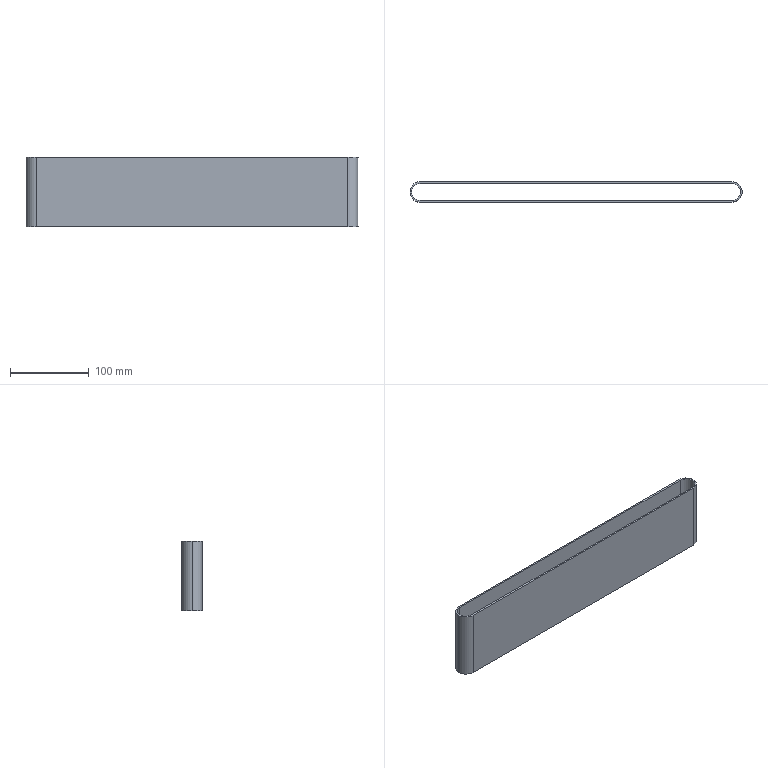Part | STEP file | Red flat belt 816 | 1 solid | 12 faces | box 423 x 26 x 89 mm | volume 154753 mm3 | cylinder 6 | plane 6 | commonest cylinder face diameters 22 x3 26 x3
STEP:
#1=CARTESIAN_POINT('',(-198.5,11.,89.));
#2=VERTEX_POINT('',#1);
#3=CARTESIAN_POINT('',(-209.5,0.,89.));
#4=VERTEX_POINT('',#3);
#5=CARTESIAN_POINT('',(-198.5,0.,89.));
#6=DIRECTION('',(0.,0.,1.));
#7=DIRECTION('',(1.,0.,0.));
#8=AXIS2_PLACEMENT_3D('',#5,#6,#7);
#9=CIRCLE('',#8,11.);
#10=EDGE_CURVE('',#2,#4,#9,.T.);
#11=ORIENTED_EDGE('',*,*,#10,.T.);
#12=CARTESIAN_POINT('',(-209.5,0.,0.));
#13=VERTEX_POINT('',#12);
#14=CARTESIAN_POINT('',(-209.5,0.,89.));
#15=DIRECTION('',(0.,0.,-1.));
#16=VECTOR('',#15,1000.);
#17=LINE('',#14,#16);
#18=EDGE_CURVE('',#4,#13,#17,.T.);
#19=ORIENTED_EDGE('',*,*,#18,.T.);
#20=CARTESIAN_POINT('',(-198.5,11.,0.));
#21=VERTEX_POINT('',#20);
#22=CARTESIAN_POINT('',(-198.5,0.,0.));
#23=DIRECTION('',(0.,0.,1.));
#24=DIRECTION('',(1.,0.,0.));
#25=AXIS2_PLACEMENT_3D('',#22,#23,#24);
#26=CIRCLE('',#25,11.);
#27=EDGE_CURVE('',#21,#13,#26,.T.);
#28=ORIENTED_EDGE('',*,*,#27,.F.);
#29=CARTESIAN_POINT('',(-198.5,11.,89.));
#30=DIRECTION('',(0.,0.,-1.));
#31=VECTOR('',#30,1000.);
#32=LINE('',#29,#31);
#33=EDGE_CURVE('',#2,#21,#32,.T.);
#34=ORIENTED_EDGE('',*,*,#33,.F.);
#35=EDGE_LOOP('',(#11,#19,#28,#34));
#36=FACE_OUTER_BOUND('',#35,.T.);
#37=CARTESIAN_POINT('',(-198.5,0.,89.));
#38=DIRECTION('',(0.,0.,-1.));
#39=DIRECTION('',(-1.,0.,0.));
#40=AXIS2_PLACEMENT_3D('',#37,#38,#39);
#41=CYLINDRICAL_SURFACE('',#40,11.);
#42=ADVANCED_FACE('',(#36),#41,.F.);
#43=CARTESIAN_POINT('',(-211.5,0.,89.));
#44=VERTEX_POINT('',#43);
#45=CARTESIAN_POINT('',(-198.5,-13.,89.));
#46=VERTEX_POINT('',#45);
#47=CARTESIAN_POINT('',(-198.5,0.,89.));
#48=DIRECTION('',(0.,0.,1.));
#49=DIRECTION('',(1.,0.,0.));
#50=AXIS2_PLACEMENT_3D('',#47,#48,#49);
#51=CIRCLE('',#50,13.);
#52=EDGE_CURVE('',#44,#46,#51,.T.);
#53=ORIENTED_EDGE('',*,*,#52,.F.);
#54=CARTESIAN_POINT('',(-211.5,0.,0.));
#55=VERTEX_POINT('',#54);
#56=CARTESIAN_POINT('',(-211.5,0.,89.));
#57=DIRECTION('',(0.,0.,-1.));
#58=VECTOR('',#57,1000.);
#59=LINE('',#56,#58);
#60=EDGE_CURVE('',#44,#55,#59,.T.);
#61=ORIENTED_EDGE('',*,*,#60,.T.);
#62=CARTESIAN_POINT('',(-198.5,-13.,0.));
#63=VERTEX_POINT('',#62);
#64=CARTESIAN_POINT('',(-198.5,0.,0.));
#65=DIRECTION('',(0.,0.,1.));
#66=DIRECTION('',(1.,0.,0.));
#67=AXIS2_PLACEMENT_3D('',#64,#65,#66);
#68=CIRCLE('',#67,13.);
#69=EDGE_CURVE('',#55,#63,#68,.T.);
#70=ORIENTED_EDGE('',*,*,#69,.T.);
#71=CARTESIAN_POINT('',(-198.5,-13.,89.));
#72=DIRECTION('',(0.,0.,-1.));
#73=VECTOR('',#72,1000.);
#74=LINE('',#71,#73);
#75=EDGE_CURVE('',#46,#63,#74,.T.);
#76=ORIENTED_EDGE('',*,*,#75,.F.);
#77=EDGE_LOOP('',(#53,#61,#70,#76));
#78=FACE_OUTER_BOUND('',#77,.T.);
#79=CARTESIAN_POINT('',(-198.5,0.,89.));
#80=DIRECTION('',(0.,0.,-1.));
#81=DIRECTION('',(-1.,0.,0.));
#82=AXIS2_PLACEMENT_3D('',#79,#80,#81);
#83=CYLINDRICAL_SURFACE('',#82,13.);
#84=ADVANCED_FACE('',(#78),#83,.T.);
#85=CARTESIAN_POINT('',(-198.5,13.,89.));
#86=VERTEX_POINT('',#85);
#87=CARTESIAN_POINT('',(-198.5,0.,89.));
#88=DIRECTION('',(0.,0.,1.));
#89=DIRECTION('',(1.,0.,0.));
#90=AXIS2_PLACEMENT_3D('',#87,#88,#89);
#91=CIRCLE('',#90,13.);
#92=EDGE_CURVE('',#86,#44,#91,.T.);
#93=ORIENTED_EDGE('',*,*,#92,.T.);
#94=ORIENTED_EDGE('',*,*,#52,.T.);
#95=CARTESIAN_POINT('',(198.5,-13.,89.));
#96=VERTEX_POINT('',#95);
#97=CARTESIAN_POINT('',(-198.5,-13.,89.));
#98=DIRECTION('',(1.,0.,0.));
#99=VECTOR('',#98,1000.);
#100=LINE('',#97,#99);
#101=EDGE_CURVE('',#46,#96,#100,.T.);
#102=ORIENTED_EDGE('',*,*,#101,.T.);
#103=CARTESIAN_POINT('',(198.5,13.,89.));
#104=VERTEX_POINT('',#103);
#105=CARTESIAN_POINT('',(198.5,0.,89.));
#106=DIRECTION('',(0.,0.,1.));
#107=DIRECTION('',(1.,0.,0.));
#108=AXIS2_PLACEMENT_3D('',#105,#106,#107);
#109=CIRCLE('',#108,13.);
#110=EDGE_CURVE('',#96,#104,#109,.T.);
#111=ORIENTED_EDGE('',*,*,#110,.T.);
#112=CARTESIAN_POINT('',(-198.5,13.,89.));
#113=DIRECTION('',(-1.,0.,0.));
#114=VECTOR('',#113,1000.);
#115=LINE('',#112,#114);
#116=EDGE_CURVE('',#104,#86,#115,.T.);
#117=ORIENTED_EDGE('',*,*,#116,.T.);
#118=EDGE_LOOP('',(#93,#94,#102,#111,#117));
#119=FACE_OUTER_BOUND('',#118,.T.);
#120=CARTESIAN_POINT('',(-198.5,-11.,89.));
#121=VERTEX_POINT('',#120);
#122=CARTESIAN_POINT('',(198.5,-11.,89.));
#123=VERTEX_POINT('',#122);
#124=CARTESIAN_POINT('',(-198.5,-11.,89.));
#125=DIRECTION('',(1.,0.,0.));
#126=VECTOR('',#125,1000.);
#127=LINE('',#124,#126);
#128=EDGE_CURVE('',#121,#123,#127,.T.);
#129=ORIENTED_EDGE('',*,*,#128,.F.);
#130=CARTESIAN_POINT('',(-198.5,0.,89.));
#131=DIRECTION('',(0.,0.,1.));
#132=DIRECTION('',(1.,0.,0.));
#133=AXIS2_PLACEMENT_3D('',#130,#131,#132);
#134=CIRCLE('',#133,11.);
#135=EDGE_CURVE('',#4,#121,#134,.T.);
#136=ORIENTED_EDGE('',*,*,#135,.F.);
#137=ORIENTED_EDGE('',*,*,#10,.F.);
#138=CARTESIAN_POINT('',(198.5,11.,89.));
#139=VERTEX_POINT('',#138);
#140=CARTESIAN_POINT('',(-198.5,11.,89.));
#141=DIRECTION('',(-1.,0.,0.));
#142=VECTOR('',#141,1000.);
#143=LINE('',#140,#142);
#144=EDGE_CURVE('',#139,#2,#143,.T.);
#145=ORIENTED_EDGE('',*,*,#144,.F.);
#146=CARTESIAN_POINT('',(198.5,0.,89.));
#147=DIRECTION('',(0.,0.,1.));
#148=DIRECTION('',(1.,0.,0.));
#149=AXIS2_PLACEMENT_3D('',#146,#147,#148);
#150=CIRCLE('',#149,11.);
#151=EDGE_CURVE('',#123,#139,#150,.T.);
#152=ORIENTED_EDGE('',*,*,#151,.F.);
#153=EDGE_LOOP('',(#129,#136,#137,#145,#152));
#154=FACE_BOUND('',#153,.T.);
#155=CARTESIAN_POINT('',(-198.5,0.,89.));
#156=DIRECTION('',(0.,0.,1.));
#157=DIRECTION('',(1.,0.,0.));
#158=AXIS2_PLACEMENT_3D('',#155,#156,#157);
#159=PLANE('',#158);
#160=ADVANCED_FACE('',(#119,#154),#159,.T.);
#161=CARTESIAN_POINT('',(-198.5,13.,0.));
#162=VERTEX_POINT('',#161);
#163=CARTESIAN_POINT('',(-198.5,0.,0.));
#164=DIRECTION('',(0.,0.,1.));
#165=DIRECTION('',(1.,0.,0.));
#166=AXIS2_PLACEMENT_3D('',#163,#164,#165);
#167=CIRCLE('',#166,13.);
#168=EDGE_CURVE('',#162,#55,#167,.T.);
#169=ORIENTED_EDGE('',*,*,#168,.F.);
#170=CARTESIAN_POINT('',(198.5,13.,0.));
#171=VERTEX_POINT('',#170);
#172=CARTESIAN_POINT('',(-198.5,13.,0.));
#173=DIRECTION('',(-1.,0.,0.));
#174=VECTOR('',#173,1000.);
#175=LINE('',#172,#174);
#176=EDGE_CURVE('',#171,#162,#175,.T.);
#177=ORIENTED_EDGE('',*,*,#176,.F.);
#178=CARTESIAN_POINT('',(198.5,-13.,0.));
#179=VERTEX_POINT('',#178);
#180=CARTESIAN_POINT('',(198.5,0.,0.));
#181=DIRECTION('',(0.,0.,1.));
#182=DIRECTION('',(1.,0.,0.));
#183=AXIS2_PLACEMENT_3D('',#180,#181,#182);
#184=CIRCLE('',#183,13.);
#185=EDGE_CURVE('',#179,#171,#184,.T.);
#186=ORIENTED_EDGE('',*,*,#185,.F.);
#187=CARTESIAN_POINT('',(-198.5,-13.,0.));
#188=DIRECTION('',(1.,0.,0.));
#189=VECTOR('',#188,1000.);
#190=LINE('',#187,#189);
#191=EDGE_CURVE('',#63,#179,#190,.T.);
#192=ORIENTED_EDGE('',*,*,#191,.F.);
#193=ORIENTED_EDGE('',*,*,#69,.F.);
#194=EDGE_LOOP('',(#169,#177,#186,#192,#193));
#195=FACE_OUTER_BOUND('',#194,.T.);
#196=ORIENTED_EDGE('',*,*,#27,.T.);
#197=CARTESIAN_POINT('',(-198.5,-11.,0.));
#198=VERTEX_POINT('',#197);
#199=CARTESIAN_POINT('',(-198.5,0.,0.));
#200=DIRECTION('',(0.,0.,1.));
#201=DIRECTION('',(1.,0.,0.));
#202=AXIS2_PLACEMENT_3D('',#199,#200,#201);
#203=CIRCLE('',#202,11.);
#204=EDGE_CURVE('',#13,#198,#203,.T.);
#205=ORIENTED_EDGE('',*,*,#204,.T.);
#206=CARTESIAN_POINT('',(198.5,-11.,0.));
#207=VERTEX_POINT('',#206);
#208=CARTESIAN_POINT('',(-198.5,-11.,0.));
#209=DIRECTION('',(1.,0.,0.));
#210=VECTOR('',#209,1000.);
#211=LINE('',#208,#210);
#212=EDGE_CURVE('',#198,#207,#211,.T.);
#213=ORIENTED_EDGE('',*,*,#212,.T.);
#214=CARTESIAN_POINT('',(198.5,11.,0.));
#215=VERTEX_POINT('',#214);
#216=CARTESIAN_POINT('',(198.5,0.,0.));
#217=DIRECTION('',(0.,0.,1.));
#218=DIRECTION('',(1.,0.,0.));
#219=AXIS2_PLACEMENT_3D('',#216,#217,#218);
#220=CIRCLE('',#219,11.);
#221=EDGE_CURVE('',#207,#215,#220,.T.);
#222=ORIENTED_EDGE('',*,*,#221,.T.);
#223=CARTESIAN_POINT('',(-198.5,11.,0.));
#224=DIRECTION('',(-1.,0.,0.));
#225=VECTOR('',#224,1000.);
#226=LINE('',#223,#225);
#227=EDGE_CURVE('',#215,#21,#226,.T.);
#228=ORIENTED_EDGE('',*,*,#227,.T.);
#229=EDGE_LOOP('',(#196,#205,#213,#222,#228));
#230=FACE_BOUND('',#229,.T.);
#231=CARTESIAN_POINT('',(-198.5,0.,0.));
#232=DIRECTION('',(0.,0.,1.));
#233=DIRECTION('',(1.,0.,0.));
#234=AXIS2_PLACEMENT_3D('',#231,#232,#233);
#235=PLANE('',#234);
#236=ADVANCED_FACE('',(#195,#230),#235,.F.);
#237=ORIENTED_EDGE('',*,*,#60,.F.);
#238=ORIENTED_EDGE('',*,*,#92,.F.);
#239=CARTESIAN_POINT('',(-198.5,13.,89.));
#240=DIRECTION('',(0.,0.,-1.));
#241=VECTOR('',#240,1000.);
#242=LINE('',#239,#241);
#243=EDGE_CURVE('',#86,#162,#242,.T.);
#244=ORIENTED_EDGE('',*,*,#243,.T.);
#245=ORIENTED_EDGE('',*,*,#168,.T.);
#246=EDGE_LOOP('',(#237,#238,#244,#245));
#247=FACE_OUTER_BOUND('',#246,.T.);
#248=CARTESIAN_POINT('',(-198.5,0.,89.));
#249=DIRECTION('',(0.,0.,-1.));
#250=DIRECTION('',(-1.,0.,0.));
#251=AXIS2_PLACEMENT_3D('',#248,#249,#250);
#252=CYLINDRICAL_SURFACE('',#251,13.);
#253=ADVANCED_FACE('',(#247),#252,.T.);
#254=ORIENTED_EDGE('',*,*,#191,.T.);
#255=CARTESIAN_POINT('',(198.5,-13.,89.));
#256=DIRECTION('',(0.,0.,-1.));
#257=VECTOR('',#256,1000.);
#258=LINE('',#255,#257);
#259=EDGE_CURVE('',#96,#179,#258,.T.);
#260=ORIENTED_EDGE('',*,*,#259,.F.);
#261=ORIENTED_EDGE('',*,*,#101,.F.);
#262=ORIENTED_EDGE('',*,*,#75,.T.);
#263=EDGE_LOOP('',(#254,#260,#261,#262));
#264=FACE_OUTER_BOUND('',#263,.T.);
#265=CARTESIAN_POINT('',(-198.5,-13.,89.));
#266=DIRECTION('',(0.,1.,0.));
#267=DIRECTION('',(-1.,0.,0.));
#268=AXIS2_PLACEMENT_3D('',#265,#266,#267);
#269=PLANE('',#268);
#270=ADVANCED_FACE('',(#264),#269,.F.);
#271=ORIENTED_EDGE('',*,*,#185,.T.);
#272=CARTESIAN_POINT('',(198.5,13.,89.));
#273=DIRECTION('',(0.,0.,-1.));
#274=VECTOR('',#273,1000.);
#275=LINE('',#272,#274);
#276=EDGE_CURVE('',#104,#171,#275,.T.);
#277=ORIENTED_EDGE('',*,*,#276,.F.);
#278=ORIENTED_EDGE('',*,*,#110,.F.);
#279=ORIENTED_EDGE('',*,*,#259,.T.);
#280=EDGE_LOOP('',(#271,#277,#278,#279));
#281=FACE_OUTER_BOUND('',#280,.T.);
#282=CARTESIAN_POINT('',(198.5,0.,89.));
#283=DIRECTION('',(0.,0.,-1.));
#284=DIRECTION('',(-1.,0.,0.));
#285=AXIS2_PLACEMENT_3D('',#282,#283,#284);
#286=CYLINDRICAL_SURFACE('',#285,13.);
#287=ADVANCED_FACE('',(#281),#286,.T.);
#288=ORIENTED_EDGE('',*,*,#176,.T.);
#289=ORIENTED_EDGE('',*,*,#243,.F.);
#290=ORIENTED_EDGE('',*,*,#116,.F.);
#291=ORIENTED_EDGE('',*,*,#276,.T.);
#292=EDGE_LOOP('',(#288,#289,#290,#291));
#293=FACE_OUTER_BOUND('',#292,.T.);
#294=CARTESIAN_POINT('',(-198.5,13.,89.));
#295=DIRECTION('',(0.,-1.,0.));
#296=DIRECTION('',(0.,0.,-1.));
#297=AXIS2_PLACEMENT_3D('',#294,#295,#296);
#298=PLANE('',#297);
#299=ADVANCED_FACE('',(#293),#298,.F.);
#300=ORIENTED_EDGE('',*,*,#18,.F.);
#301=ORIENTED_EDGE('',*,*,#135,.T.);
#302=CARTESIAN_POINT('',(-198.5,-11.,89.));
#303=DIRECTION('',(0.,0.,-1.));
#304=VECTOR('',#303,1000.);
#305=LINE('',#302,#304);
#306=EDGE_CURVE('',#121,#198,#305,.T.);
#307=ORIENTED_EDGE('',*,*,#306,.T.);
#308=ORIENTED_EDGE('',*,*,#204,.F.);
#309=EDGE_LOOP('',(#300,#301,#307,#308));
#310=FACE_OUTER_BOUND('',#309,.T.);
#311=CARTESIAN_POINT('',(-198.5,0.,89.));
#312=DIRECTION('',(0.,0.,-1.));
#313=DIRECTION('',(-1.,0.,0.));
#314=AXIS2_PLACEMENT_3D('',#311,#312,#313);
#315=CYLINDRICAL_SURFACE('',#314,11.);
#316=ADVANCED_FACE('',(#310),#315,.F.);
#317=ORIENTED_EDGE('',*,*,#212,.F.);
#318=ORIENTED_EDGE('',*,*,#306,.F.);
#319=ORIENTED_EDGE('',*,*,#128,.T.);
#320=CARTESIAN_POINT('',(198.5,-11.,89.));
#321=DIRECTION('',(0.,0.,-1.));
#322=VECTOR('',#321,1000.);
#323=LINE('',#320,#322);
#324=EDGE_CURVE('',#123,#207,#323,.T.);
#325=ORIENTED_EDGE('',*,*,#324,.T.);
#326=EDGE_LOOP('',(#317,#318,#319,#325));
#327=FACE_OUTER_BOUND('',#326,.T.);
#328=CARTESIAN_POINT('',(-198.5,-11.,89.));
#329=DIRECTION('',(0.,1.,0.));
#330=DIRECTION('',(-1.,0.,0.));
#331=AXIS2_PLACEMENT_3D('',#328,#329,#330);
#332=PLANE('',#331);
#333=ADVANCED_FACE('',(#327),#332,.T.);
#334=ORIENTED_EDGE('',*,*,#221,.F.);
#335=ORIENTED_EDGE('',*,*,#324,.F.);
#336=ORIENTED_EDGE('',*,*,#151,.T.);
#337=CARTESIAN_POINT('',(198.5,11.,89.));
#338=DIRECTION('',(0.,0.,-1.));
#339=VECTOR('',#338,1000.);
#340=LINE('',#337,#339);
#341=EDGE_CURVE('',#139,#215,#340,.T.);
#342=ORIENTED_EDGE('',*,*,#341,.T.);
#343=EDGE_LOOP('',(#334,#335,#336,#342));
#344=FACE_OUTER_BOUND('',#343,.T.);
#345=CARTESIAN_POINT('',(198.5,0.,89.));
#346=DIRECTION('',(0.,0.,-1.));
#347=DIRECTION('',(-1.,0.,0.));
#348=AXIS2_PLACEMENT_3D('',#345,#346,#347);
#349=CYLINDRICAL_SURFACE('',#348,11.);
#350=ADVANCED_FACE('',(#344),#349,.F.);
#351=ORIENTED_EDGE('',*,*,#227,.F.);
#352=ORIENTED_EDGE('',*,*,#341,.F.);
#353=ORIENTED_EDGE('',*,*,#144,.T.);
#354=ORIENTED_EDGE('',*,*,#33,.T.);
#355=EDGE_LOOP('',(#351,#352,#353,#354));
#356=FACE_OUTER_BOUND('',#355,.T.);
#357=CARTESIAN_POINT('',(-198.5,11.,89.));
#358=DIRECTION('',(0.,-1.,0.));
#359=DIRECTION('',(1.,0.,0.));
#360=AXIS2_PLACEMENT_3D('',#357,#358,#359);
#361=PLANE('',#360);
#362=ADVANCED_FACE('',(#356),#361,.T.);
#363=CLOSED_SHELL('',(#42,#84,#160,#236,#253,#270,#287,#299,#316,#333,#350,#362));
#364=MANIFOLD_SOLID_BREP('',#363);
#365=CARTESIAN_POINT('',(0.,0.,0.));
#366=DIRECTION('',(0.,0.,1.));
#367=DIRECTION('',(1.,0.,0.));
#368=AXIS2_PLACEMENT_3D('',#365,#366,#367);
#369=(LENGTH_UNIT()NAMED_UNIT(*)SI_UNIT(.MILLI.,.METRE.));
#370=UNCERTAINTY_MEASURE_WITH_UNIT(LENGTH_MEASURE(0.00001),#369,'','');
#371=(NAMED_UNIT(*)PLANE_ANGLE_UNIT()SI_UNIT($,.RADIAN.));
#372=(NAMED_UNIT(*)SI_UNIT($,.STERADIAN.)SOLID_ANGLE_UNIT());
#373=(GEOMETRIC_REPRESENTATION_CONTEXT(3)GLOBAL_UNCERTAINTY_ASSIGNED_CONTEXT((#370))GLOBAL_UNIT_ASSIGNED_CONTEXT((#369,#371,#372))REPRESENTATION_CONTEXT('',''));
#374=ADVANCED_BREP_SHAPE_REPRESENTATION('',(#364,#368),#373);